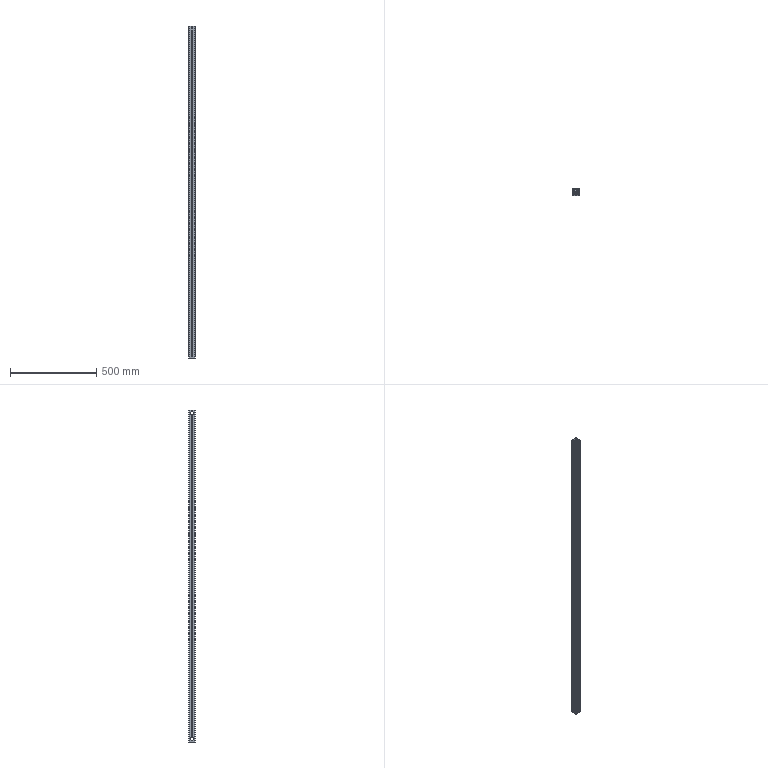Part | SolidWorks | features BaseBody 1, HoleWzd 1, MoveFace 1 | 1 solid | 242 faces | box 40 x 40 x 1920 mm | volume 1128397 mm3 | plane 187 | cylinder 55 | commonest cylinder face diameters 6.8 x15 2 x14 19 x12 1 x6 5 x4 9 x4